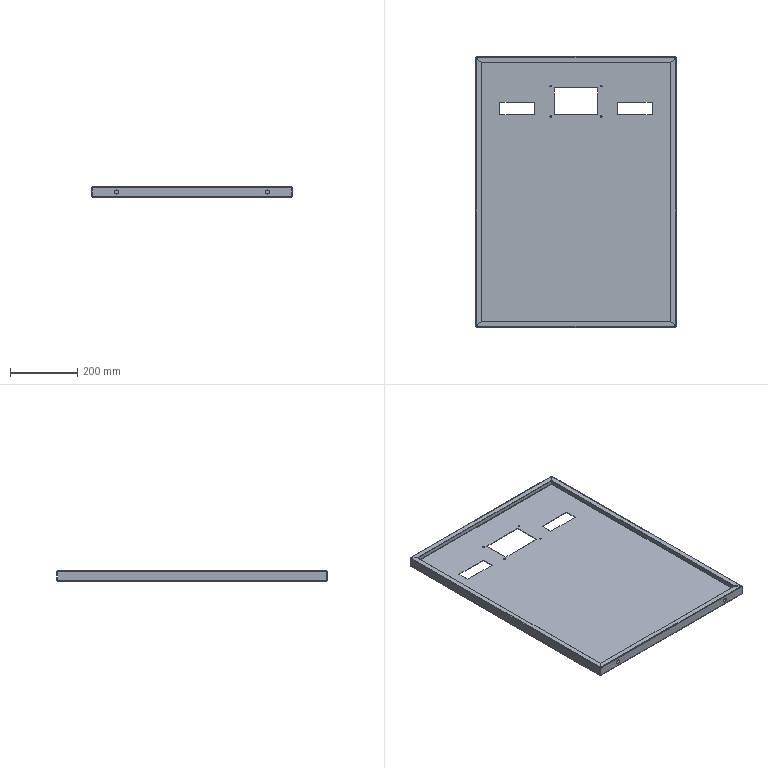Part | NX | 1 solid | 88 faces | box 598 x 804 x 30 mm | volume 868795 mm3 | plane 50 | cylinder 22 | spline 16 | commonest cylinder face diameters 1.473 x8 4.473 x8 4.8 x4 12 x2